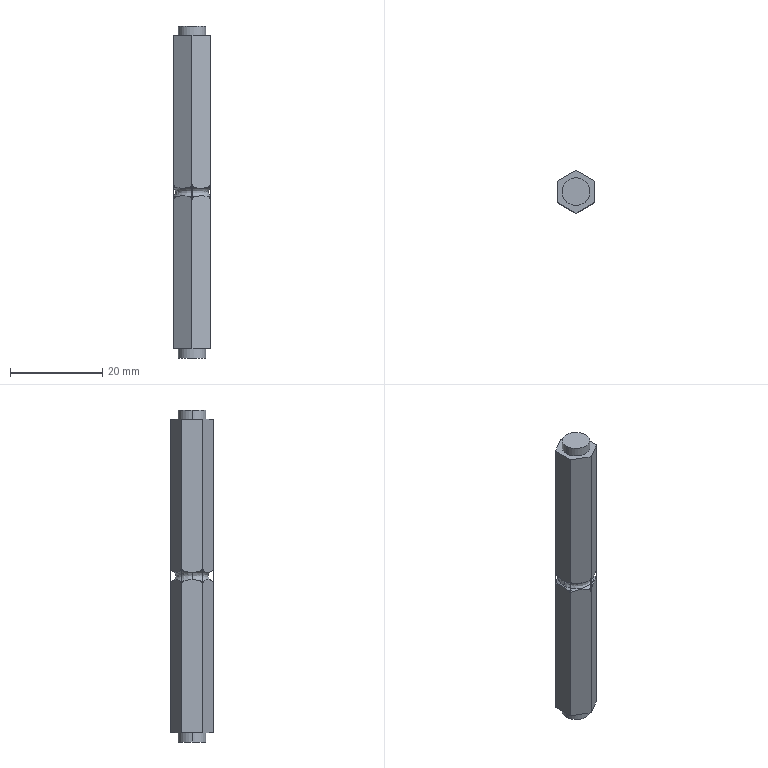Part | STEP file | 1 solid | 38 faces | box 8 x 9.238 x 72 mm | volume 3859 mm3 | spline 14 | cylinder 10 | plane 10 | cone 4 | commonest cylinder face diameters 9.214 x6 6 x4